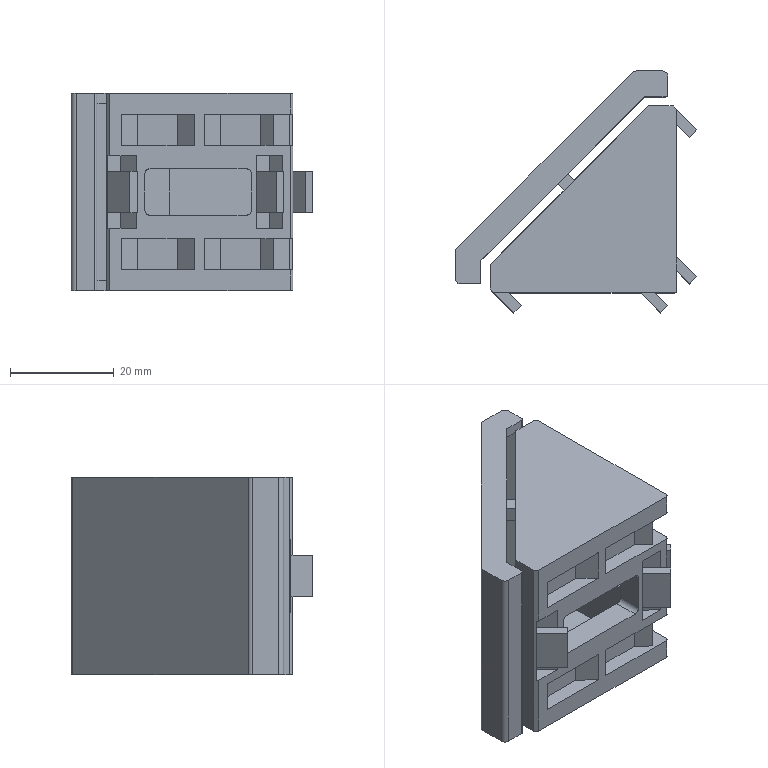Part | SolidWorks | 1 solid | 164 faces | box 46.643 x 46.639 x 38 mm | volume 6782 mm3 | plane 130 | cylinder 32 | cone 2 | commonest cylinder face diameters 2 x21 1 x7 1.72 x4